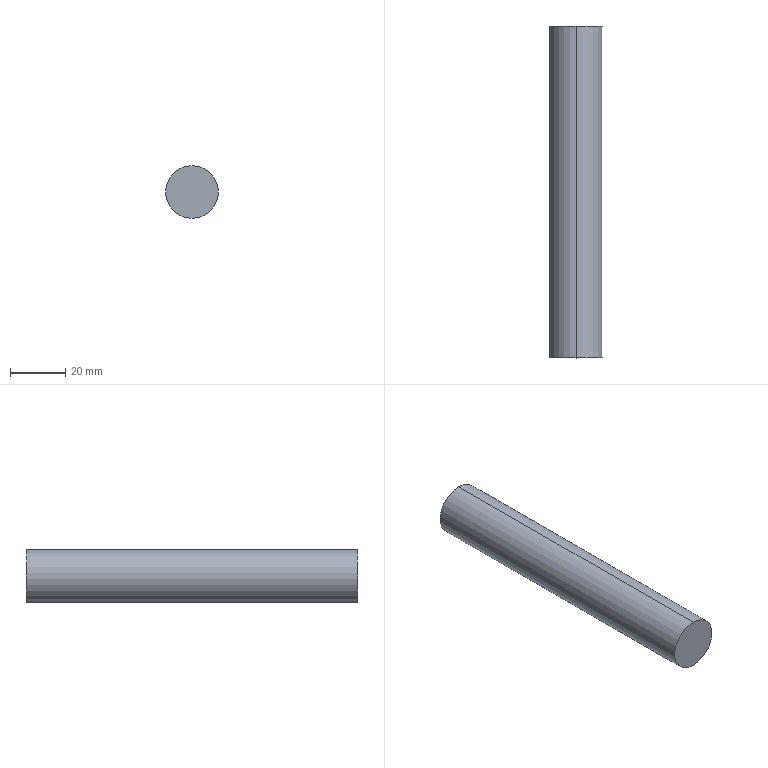Part | STEP file | 1 solid | 4 faces | box 19 x 120 x 19 mm | volume 34023 mm3 | cylinder 2 | plane 2 | commonest cylinder face diameters 19 x2
STEP:
#1=CARTESIAN_POINT('',(0.,0.,0.));
#2=DIRECTION('',(0.,0.,1.));
#3=DIRECTION('',(1.,0.,0.));
#4=AXIS2_PLACEMENT_3D('',#1,#2,#3);
#5=CARTESIAN_POINT('',(0.,120.,9.5));
#6=VERTEX_POINT('',#5);
#7=CARTESIAN_POINT('',(0.,120.,-9.5));
#8=VERTEX_POINT('',#7);
#9=CARTESIAN_POINT('',(0.,120.,0.));
#10=DIRECTION('',(0.,1.,0.));
#11=DIRECTION('',(0.,0.,1.));
#12=AXIS2_PLACEMENT_3D('',#9,#10,#11);
#13=CIRCLE('',#12,9.5);
#14=CARTESIAN_POINT('',(0.,120.,0.));
#15=DIRECTION('',(0.,-1.,0.));
#16=DIRECTION('',(0.,0.,-1.));
#17=AXIS2_PLACEMENT_3D('',#14,#15,#16);
#18=CYLINDRICAL_SURFACE('',#17,9.5);
#19=CARTESIAN_POINT('',(3.142,0.));
#20=DIRECTION('',(-1.,0.));
#21=VECTOR('',#20,1.);
#22=LINE('',#19,#21);
#23=(GEOMETRIC_REPRESENTATION_CONTEXT(2)PARAMETRIC_REPRESENTATION_CONTEXT()REPRESENTATION_CONTEXT('',''));
#24=DEFINITIONAL_REPRESENTATION('',(#22),#23);
#25=PCURVE('',#18,#24);
#26=CARTESIAN_POINT('',(0.,120.,0.));
#27=DIRECTION('',(0.,1.,0.));
#28=DIRECTION('',(0.,0.,1.));
#29=AXIS2_PLACEMENT_3D('',#26,#27,#28);
#30=PLANE('',#29);
#31=CARTESIAN_POINT('',(0.,0.));
#32=DIRECTION('',(1.,0.));
#33=AXIS2_PLACEMENT_2D('',#31,#32);
#34=CIRCLE('',#33,9.5);
#35=(GEOMETRIC_REPRESENTATION_CONTEXT(2)PARAMETRIC_REPRESENTATION_CONTEXT()REPRESENTATION_CONTEXT('',''));
#36=DEFINITIONAL_REPRESENTATION('',(#34),#35);
#37=PCURVE('',#30,#36);
#38=SURFACE_CURVE('',#13,(#25,#37),.PCURVE_S1.);
#39=EDGE_CURVE('',#6,#8,#38,.T.);
#40=ORIENTED_EDGE('',*,*,#39,.F.);
#41=CARTESIAN_POINT('',(0.,0.,9.5));
#42=VERTEX_POINT('',#41);
#43=CARTESIAN_POINT('',(0.,120.,9.5));
#44=DIRECTION('',(0.,-1.,0.));
#45=VECTOR('',#44,1.);
#46=LINE('',#43,#45);
#47=CARTESIAN_POINT('',(3.142,0.));
#48=DIRECTION('',(0.,1.));
#49=VECTOR('',#48,1.);
#50=LINE('',#47,#49);
#51=(GEOMETRIC_REPRESENTATION_CONTEXT(2)PARAMETRIC_REPRESENTATION_CONTEXT()REPRESENTATION_CONTEXT('',''));
#52=DEFINITIONAL_REPRESENTATION('',(#50),#51);
#53=PCURVE('',#18,#52);
#54=CARTESIAN_POINT('',(0.,120.,0.));
#55=DIRECTION('',(0.,-1.,0.));
#56=DIRECTION('',(0.,0.,-1.));
#57=AXIS2_PLACEMENT_3D('',#54,#55,#56);
#58=CYLINDRICAL_SURFACE('',#57,9.5);
#59=CARTESIAN_POINT('',(3.142,0.));
#60=DIRECTION('',(0.,1.));
#61=VECTOR('',#60,1.);
#62=LINE('',#59,#61);
#63=(GEOMETRIC_REPRESENTATION_CONTEXT(2)PARAMETRIC_REPRESENTATION_CONTEXT()REPRESENTATION_CONTEXT('',''));
#64=DEFINITIONAL_REPRESENTATION('',(#62),#63);
#65=PCURVE('',#58,#64);
#66=SURFACE_CURVE('',#46,(#53,#65),.PCURVE_S1.);
#67=EDGE_CURVE('',#6,#42,#66,.T.);
#68=ORIENTED_EDGE('',*,*,#67,.T.);
#69=CARTESIAN_POINT('',(0.,0.,-9.5));
#70=VERTEX_POINT('',#69);
#71=CARTESIAN_POINT('',(0.,0.,0.));
#72=DIRECTION('',(0.,1.,0.));
#73=DIRECTION('',(0.,0.,1.));
#74=AXIS2_PLACEMENT_3D('',#71,#72,#73);
#75=CIRCLE('',#74,9.5);
#76=CARTESIAN_POINT('',(3.142,120.));
#77=DIRECTION('',(-1.,0.));
#78=VECTOR('',#77,1.);
#79=LINE('',#76,#78);
#80=(GEOMETRIC_REPRESENTATION_CONTEXT(2)PARAMETRIC_REPRESENTATION_CONTEXT()REPRESENTATION_CONTEXT('',''));
#81=DEFINITIONAL_REPRESENTATION('',(#79),#80);
#82=PCURVE('',#18,#81);
#83=CARTESIAN_POINT('',(0.,0.,0.));
#84=DIRECTION('',(0.,1.,0.));
#85=DIRECTION('',(0.,0.,1.));
#86=AXIS2_PLACEMENT_3D('',#83,#84,#85);
#87=PLANE('',#86);
#88=CARTESIAN_POINT('',(0.,0.));
#89=DIRECTION('',(1.,0.));
#90=AXIS2_PLACEMENT_2D('',#88,#89);
#91=CIRCLE('',#90,9.5);
#92=(GEOMETRIC_REPRESENTATION_CONTEXT(2)PARAMETRIC_REPRESENTATION_CONTEXT()REPRESENTATION_CONTEXT('',''));
#93=DEFINITIONAL_REPRESENTATION('',(#91),#92);
#94=PCURVE('',#87,#93);
#95=SURFACE_CURVE('',#75,(#82,#94),.PCURVE_S1.);
#96=EDGE_CURVE('',#42,#70,#95,.T.);
#97=ORIENTED_EDGE('',*,*,#96,.T.);
#98=CARTESIAN_POINT('',(0.,120.,-9.5));
#99=DIRECTION('',(0.,-1.,0.));
#100=VECTOR('',#99,1.);
#101=LINE('',#98,#100);
#102=CARTESIAN_POINT('',(0.,0.));
#103=DIRECTION('',(0.,1.));
#104=VECTOR('',#103,1.);
#105=LINE('',#102,#104);
#106=(GEOMETRIC_REPRESENTATION_CONTEXT(2)PARAMETRIC_REPRESENTATION_CONTEXT()REPRESENTATION_CONTEXT('',''));
#107=DEFINITIONAL_REPRESENTATION('',(#105),#106);
#108=PCURVE('',#18,#107);
#109=CARTESIAN_POINT('',(6.283,0.));
#110=DIRECTION('',(0.,1.));
#111=VECTOR('',#110,1.);
#112=LINE('',#109,#111);
#113=(GEOMETRIC_REPRESENTATION_CONTEXT(2)PARAMETRIC_REPRESENTATION_CONTEXT()REPRESENTATION_CONTEXT('',''));
#114=DEFINITIONAL_REPRESENTATION('',(#112),#113);
#115=PCURVE('',#58,#114);
#116=SURFACE_CURVE('',#101,(#108,#115),.PCURVE_S1.);
#117=EDGE_CURVE('',#8,#70,#116,.T.);
#118=ORIENTED_EDGE('',*,*,#117,.F.);
#119=EDGE_LOOP('',(#40,#68,#97,#118));
#120=FACE_BOUND('',#119,.T.);
#121=ADVANCED_FACE('',(#120),#18,.T.);
#122=ORIENTED_EDGE('',*,*,#67,.F.);
#123=CARTESIAN_POINT('',(0.,120.,0.));
#124=DIRECTION('',(0.,1.,0.));
#125=DIRECTION('',(0.,0.,1.));
#126=AXIS2_PLACEMENT_3D('',#123,#124,#125);
#127=CIRCLE('',#126,9.5);
#128=CARTESIAN_POINT('',(9.425,0.));
#129=DIRECTION('',(-1.,0.));
#130=VECTOR('',#129,1.);
#131=LINE('',#128,#130);
#132=(GEOMETRIC_REPRESENTATION_CONTEXT(2)PARAMETRIC_REPRESENTATION_CONTEXT()REPRESENTATION_CONTEXT('',''));
#133=DEFINITIONAL_REPRESENTATION('',(#131),#132);
#134=PCURVE('',#58,#133);
#135=CARTESIAN_POINT('',(0.,0.));
#136=DIRECTION('',(1.,0.));
#137=AXIS2_PLACEMENT_2D('',#135,#136);
#138=CIRCLE('',#137,9.5);
#139=(GEOMETRIC_REPRESENTATION_CONTEXT(2)PARAMETRIC_REPRESENTATION_CONTEXT()REPRESENTATION_CONTEXT('',''));
#140=DEFINITIONAL_REPRESENTATION('',(#138),#139);
#141=PCURVE('',#30,#140);
#142=SURFACE_CURVE('',#127,(#134,#141),.PCURVE_S1.);
#143=EDGE_CURVE('',#8,#6,#142,.T.);
#144=ORIENTED_EDGE('',*,*,#143,.F.);
#145=ORIENTED_EDGE('',*,*,#117,.T.);
#146=CARTESIAN_POINT('',(0.,0.,0.));
#147=DIRECTION('',(0.,1.,0.));
#148=DIRECTION('',(0.,0.,1.));
#149=AXIS2_PLACEMENT_3D('',#146,#147,#148);
#150=CIRCLE('',#149,9.5);
#151=CARTESIAN_POINT('',(9.425,120.));
#152=DIRECTION('',(-1.,0.));
#153=VECTOR('',#152,1.);
#154=LINE('',#151,#153);
#155=(GEOMETRIC_REPRESENTATION_CONTEXT(2)PARAMETRIC_REPRESENTATION_CONTEXT()REPRESENTATION_CONTEXT('',''));
#156=DEFINITIONAL_REPRESENTATION('',(#154),#155);
#157=PCURVE('',#58,#156);
#158=CARTESIAN_POINT('',(0.,0.));
#159=DIRECTION('',(1.,0.));
#160=AXIS2_PLACEMENT_2D('',#158,#159);
#161=CIRCLE('',#160,9.5);
#162=(GEOMETRIC_REPRESENTATION_CONTEXT(2)PARAMETRIC_REPRESENTATION_CONTEXT()REPRESENTATION_CONTEXT('',''));
#163=DEFINITIONAL_REPRESENTATION('',(#161),#162);
#164=PCURVE('',#87,#163);
#165=SURFACE_CURVE('',#150,(#157,#164),.PCURVE_S1.);
#166=EDGE_CURVE('',#70,#42,#165,.T.);
#167=ORIENTED_EDGE('',*,*,#166,.T.);
#168=EDGE_LOOP('',(#122,#144,#145,#167));
#169=FACE_BOUND('',#168,.T.);
#170=ADVANCED_FACE('',(#169),#58,.T.);
#171=ORIENTED_EDGE('',*,*,#143,.T.);
#172=ORIENTED_EDGE('',*,*,#39,.T.);
#173=EDGE_LOOP('',(#171,#172));
#174=FACE_BOUND('',#173,.T.);
#175=ADVANCED_FACE('',(#174),#30,.T.);
#176=ORIENTED_EDGE('',*,*,#166,.F.);
#177=ORIENTED_EDGE('',*,*,#96,.F.);
#178=EDGE_LOOP('',(#176,#177));
#179=FACE_BOUND('',#178,.T.);
#180=ADVANCED_FACE('',(#179),#87,.F.);
#181=CLOSED_SHELL('',(#121,#170,#175,#180));
#182=MANIFOLD_SOLID_BREP('',#181);
#183=(LENGTH_UNIT()NAMED_UNIT(*)SI_UNIT(.MILLI.,.METRE.));
#184=UNCERTAINTY_MEASURE_WITH_UNIT(LENGTH_MEASURE(0.0000001),#183,'','');
#185=(NAMED_UNIT(*)PLANE_ANGLE_UNIT()SI_UNIT($,.RADIAN.));
#186=(NAMED_UNIT(*)SI_UNIT($,.STERADIAN.)SOLID_ANGLE_UNIT());
#187=(GEOMETRIC_REPRESENTATION_CONTEXT(3)GLOBAL_UNCERTAINTY_ASSIGNED_CONTEXT((#184))GLOBAL_UNIT_ASSIGNED_CONTEXT((#183,#185,#186))REPRESENTATION_CONTEXT('',''));
#188=ADVANCED_BREP_SHAPE_REPRESENTATION('',(#4,#182),#187);